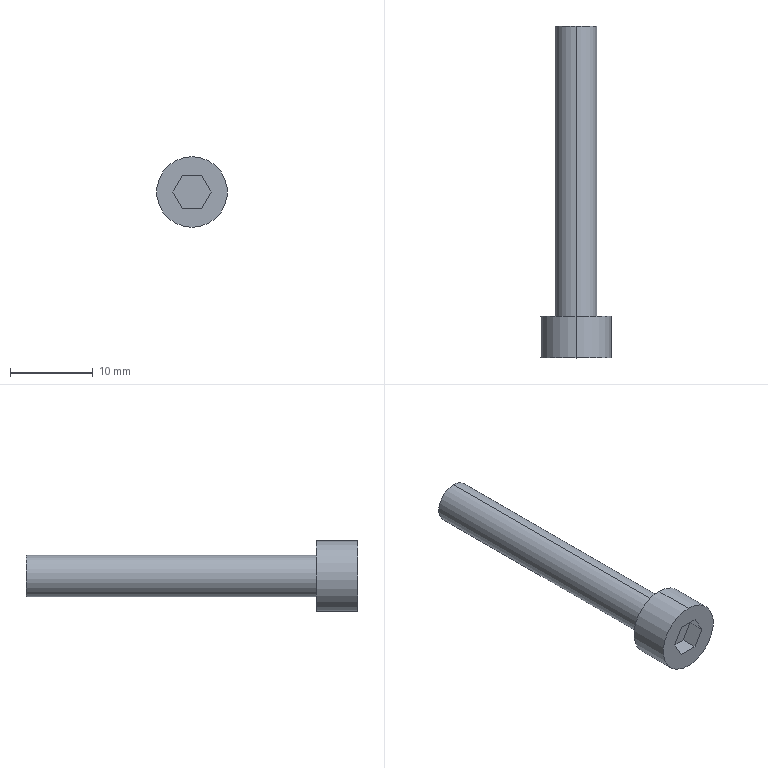Part | SolidWorks | features BaseBody 1 | 1 solid | 14 faces | box 8.5 x 40 x 8.5 mm | volume 943.236 mm3 | plane 10 | cylinder 4 | commonest cylinder face diameters 5 x2 8.5 x2
STEP:
#1=CARTESIAN_POINT('',(0.,40.,-2.5));
#2=VERTEX_POINT('',#1);
#3=CARTESIAN_POINT('',(0.,40.,2.5));
#4=VERTEX_POINT('',#3);
#5=CARTESIAN_POINT('',(0.,40.,0.));
#6=DIRECTION('',(0.,-1.,0.));
#7=DIRECTION('',(0.,0.,-1.));
#8=AXIS2_PLACEMENT_3D('',#5,#6,#7);
#9=CIRCLE('',#8,2.5);
#10=EDGE_CURVE('',#2,#4,#9,.T.);
#11=ORIENTED_EDGE('',*,*,#10,.T.);
#12=CARTESIAN_POINT('',(0.,5.,2.5));
#13=VERTEX_POINT('',#12);
#14=CARTESIAN_POINT('',(0.,40.,2.5));
#15=DIRECTION('',(0.,-1.,0.));
#16=VECTOR('',#15,1000.);
#17=LINE('',#14,#16);
#18=EDGE_CURVE('',#4,#13,#17,.T.);
#19=ORIENTED_EDGE('',*,*,#18,.T.);
#20=CARTESIAN_POINT('',(0.,5.,-2.5));
#21=VERTEX_POINT('',#20);
#22=CARTESIAN_POINT('',(0.,5.,0.));
#23=DIRECTION('',(0.,1.,0.));
#24=DIRECTION('',(0.,0.,-1.));
#25=AXIS2_PLACEMENT_3D('',#22,#23,#24);
#26=CIRCLE('',#25,2.5);
#27=EDGE_CURVE('',#13,#21,#26,.T.);
#28=ORIENTED_EDGE('',*,*,#27,.T.);
#29=CARTESIAN_POINT('',(0.,40.,-2.5));
#30=DIRECTION('',(0.,-1.,0.));
#31=VECTOR('',#30,1000.);
#32=LINE('',#29,#31);
#33=EDGE_CURVE('',#2,#21,#32,.T.);
#34=ORIENTED_EDGE('',*,*,#33,.F.);
#35=EDGE_LOOP('',(#11,#19,#28,#34));
#36=FACE_OUTER_BOUND('',#35,.T.);
#37=CARTESIAN_POINT('',(0.,40.,0.));
#38=DIRECTION('',(0.,-1.,0.));
#39=DIRECTION('',(0.,0.,-1.));
#40=AXIS2_PLACEMENT_3D('',#37,#38,#39);
#41=CYLINDRICAL_SURFACE('',#40,2.5);
#42=ADVANCED_FACE('',(#36),#41,.T.);
#43=CARTESIAN_POINT('',(0.,5.,4.25));
#44=VERTEX_POINT('',#43);
#45=CARTESIAN_POINT('',(0.,5.,-4.25));
#46=VERTEX_POINT('',#45);
#47=CARTESIAN_POINT('',(0.,5.,0.));
#48=DIRECTION('',(0.,1.,0.));
#49=DIRECTION('',(0.,0.,-1.));
#50=AXIS2_PLACEMENT_3D('',#47,#48,#49);
#51=CIRCLE('',#50,4.25);
#52=EDGE_CURVE('',#44,#46,#51,.T.);
#53=ORIENTED_EDGE('',*,*,#52,.F.);
#54=CARTESIAN_POINT('',(0.,0.,4.25));
#55=VERTEX_POINT('',#54);
#56=CARTESIAN_POINT('',(0.,5.,4.25));
#57=DIRECTION('',(0.,-1.,0.));
#58=VECTOR('',#57,1000.);
#59=LINE('',#56,#58);
#60=EDGE_CURVE('',#44,#55,#59,.T.);
#61=ORIENTED_EDGE('',*,*,#60,.T.);
#62=CARTESIAN_POINT('',(0.,0.,-4.25));
#63=VERTEX_POINT('',#62);
#64=CARTESIAN_POINT('',(0.,0.,0.));
#65=DIRECTION('',(0.,1.,0.));
#66=DIRECTION('',(0.,0.,-1.));
#67=AXIS2_PLACEMENT_3D('',#64,#65,#66);
#68=CIRCLE('',#67,4.25);
#69=EDGE_CURVE('',#55,#63,#68,.T.);
#70=ORIENTED_EDGE('',*,*,#69,.T.);
#71=CARTESIAN_POINT('',(0.,5.,-4.25));
#72=DIRECTION('',(0.,-1.,0.));
#73=VECTOR('',#72,1000.);
#74=LINE('',#71,#73);
#75=EDGE_CURVE('',#46,#63,#74,.T.);
#76=ORIENTED_EDGE('',*,*,#75,.F.);
#77=EDGE_LOOP('',(#53,#61,#70,#76));
#78=FACE_OUTER_BOUND('',#77,.T.);
#79=CARTESIAN_POINT('',(0.,5.,0.));
#80=DIRECTION('',(0.,-1.,0.));
#81=DIRECTION('',(0.,0.,-1.));
#82=AXIS2_PLACEMENT_3D('',#79,#80,#81);
#83=CYLINDRICAL_SURFACE('',#82,4.25);
#84=ADVANCED_FACE('',(#78),#83,.T.);
#85=ORIENTED_EDGE('',*,*,#18,.F.);
#86=CARTESIAN_POINT('',(0.,40.,0.));
#87=DIRECTION('',(0.,-1.,0.));
#88=DIRECTION('',(0.,0.,-1.));
#89=AXIS2_PLACEMENT_3D('',#86,#87,#88);
#90=CIRCLE('',#89,2.5);
#91=EDGE_CURVE('',#4,#2,#90,.T.);
#92=ORIENTED_EDGE('',*,*,#91,.T.);
#93=ORIENTED_EDGE('',*,*,#33,.T.);
#94=CARTESIAN_POINT('',(0.,5.,0.));
#95=DIRECTION('',(0.,1.,0.));
#96=DIRECTION('',(0.,0.,-1.));
#97=AXIS2_PLACEMENT_3D('',#94,#95,#96);
#98=CIRCLE('',#97,2.5);
#99=EDGE_CURVE('',#21,#13,#98,.T.);
#100=ORIENTED_EDGE('',*,*,#99,.T.);
#101=EDGE_LOOP('',(#85,#92,#93,#100));
#102=FACE_OUTER_BOUND('',#101,.T.);
#103=CARTESIAN_POINT('',(0.,40.,0.));
#104=DIRECTION('',(0.,-1.,0.));
#105=DIRECTION('',(0.,0.,-1.));
#106=AXIS2_PLACEMENT_3D('',#103,#104,#105);
#107=CYLINDRICAL_SURFACE('',#106,2.5);
#108=ADVANCED_FACE('',(#102),#107,.T.);
#109=CARTESIAN_POINT('',(0.,5.,0.));
#110=DIRECTION('',(0.,1.,0.));
#111=DIRECTION('',(0.,0.,-1.));
#112=AXIS2_PLACEMENT_3D('',#109,#110,#111);
#113=CIRCLE('',#112,4.25);
#114=EDGE_CURVE('',#46,#44,#113,.T.);
#115=ORIENTED_EDGE('',*,*,#114,.T.);
#116=ORIENTED_EDGE('',*,*,#52,.T.);
#117=EDGE_LOOP('',(#115,#116));
#118=FACE_OUTER_BOUND('',#117,.T.);
#119=ORIENTED_EDGE('',*,*,#99,.F.);
#120=ORIENTED_EDGE('',*,*,#27,.F.);
#121=EDGE_LOOP('',(#119,#120));
#122=FACE_BOUND('',#121,.T.);
#123=CARTESIAN_POINT('',(0.,5.,0.));
#124=DIRECTION('',(0.,1.,0.));
#125=DIRECTION('',(0.,0.,1.));
#126=AXIS2_PLACEMENT_3D('',#123,#124,#125);
#127=PLANE('',#126);
#128=ADVANCED_FACE('',(#118,#122),#127,.T.);
#129=ORIENTED_EDGE('',*,*,#10,.F.);
#130=ORIENTED_EDGE('',*,*,#91,.F.);
#131=EDGE_LOOP('',(#129,#130));
#132=FACE_OUTER_BOUND('',#131,.T.);
#133=CARTESIAN_POINT('',(0.,40.,0.));
#134=DIRECTION('',(0.,1.,0.));
#135=DIRECTION('',(0.,0.,1.));
#136=AXIS2_PLACEMENT_3D('',#133,#134,#135);
#137=PLANE('',#136);
#138=ADVANCED_FACE('',(#132),#137,.T.);
#139=ORIENTED_EDGE('',*,*,#60,.F.);
#140=ORIENTED_EDGE('',*,*,#114,.F.);
#141=ORIENTED_EDGE('',*,*,#75,.T.);
#142=CARTESIAN_POINT('',(0.,0.,0.));
#143=DIRECTION('',(0.,1.,0.));
#144=DIRECTION('',(0.,0.,-1.));
#145=AXIS2_PLACEMENT_3D('',#142,#143,#144);
#146=CIRCLE('',#145,4.25);
#147=EDGE_CURVE('',#63,#55,#146,.T.);
#148=ORIENTED_EDGE('',*,*,#147,.T.);
#149=EDGE_LOOP('',(#139,#140,#141,#148));
#150=FACE_OUTER_BOUND('',#149,.T.);
#151=CARTESIAN_POINT('',(0.,5.,0.));
#152=DIRECTION('',(0.,-1.,0.));
#153=DIRECTION('',(0.,0.,-1.));
#154=AXIS2_PLACEMENT_3D('',#151,#152,#153);
#155=CYLINDRICAL_SURFACE('',#154,4.25);
#156=ADVANCED_FACE('',(#150),#155,.T.);
#157=ORIENTED_EDGE('',*,*,#147,.F.);
#158=ORIENTED_EDGE('',*,*,#69,.F.);
#159=EDGE_LOOP('',(#157,#158));
#160=FACE_OUTER_BOUND('',#159,.T.);
#161=CARTESIAN_POINT('',(1.155,0.,-2.));
#162=VERTEX_POINT('',#161);
#163=CARTESIAN_POINT('',(2.309,0.,0.));
#164=VERTEX_POINT('',#163);
#165=CARTESIAN_POINT('',(1.155,0.,-2.));
#166=DIRECTION('',(0.5,0.,0.866));
#167=VECTOR('',#166,1000.);
#168=LINE('',#165,#167);
#169=EDGE_CURVE('',#162,#164,#168,.T.);
#170=ORIENTED_EDGE('',*,*,#169,.F.);
#171=CARTESIAN_POINT('',(-1.155,0.,-2.));
#172=VERTEX_POINT('',#171);
#173=CARTESIAN_POINT('',(0.,0.,-2.));
#174=DIRECTION('',(1.,0.,0.));
#175=VECTOR('',#174,1000.);
#176=LINE('',#173,#175);
#177=EDGE_CURVE('',#172,#162,#176,.T.);
#178=ORIENTED_EDGE('',*,*,#177,.F.);
#179=CARTESIAN_POINT('',(-2.309,0.,0.));
#180=VERTEX_POINT('',#179);
#181=CARTESIAN_POINT('',(-2.309,0.,0.));
#182=DIRECTION('',(0.5,0.,-0.866));
#183=VECTOR('',#182,1000.);
#184=LINE('',#181,#183);
#185=EDGE_CURVE('',#180,#172,#184,.T.);
#186=ORIENTED_EDGE('',*,*,#185,.F.);
#187=CARTESIAN_POINT('',(-1.155,0.,2.));
#188=VERTEX_POINT('',#187);
#189=CARTESIAN_POINT('',(-1.155,0.,2.));
#190=DIRECTION('',(-0.5,0.,-0.866));
#191=VECTOR('',#190,1000.);
#192=LINE('',#189,#191);
#193=EDGE_CURVE('',#188,#180,#192,.T.);
#194=ORIENTED_EDGE('',*,*,#193,.F.);
#195=CARTESIAN_POINT('',(1.155,0.,2.));
#196=VERTEX_POINT('',#195);
#197=CARTESIAN_POINT('',(0.,0.,2.));
#198=DIRECTION('',(-1.,0.,0.));
#199=VECTOR('',#198,1000.);
#200=LINE('',#197,#199);
#201=EDGE_CURVE('',#196,#188,#200,.T.);
#202=ORIENTED_EDGE('',*,*,#201,.F.);
#203=CARTESIAN_POINT('',(2.309,0.,0.));
#204=DIRECTION('',(-0.5,0.,0.866));
#205=VECTOR('',#204,1000.);
#206=LINE('',#203,#205);
#207=EDGE_CURVE('',#164,#196,#206,.T.);
#208=ORIENTED_EDGE('',*,*,#207,.F.);
#209=EDGE_LOOP('',(#170,#178,#186,#194,#202,#208));
#210=FACE_BOUND('',#209,.T.);
#211=CARTESIAN_POINT('',(0.,0.,0.));
#212=DIRECTION('',(0.,1.,0.));
#213=DIRECTION('',(0.,0.,1.));
#214=AXIS2_PLACEMENT_3D('',#211,#212,#213);
#215=PLANE('',#214);
#216=ADVANCED_FACE('',(#160,#210),#215,.F.);
#217=CARTESIAN_POINT('',(1.155,2.,2.));
#218=VERTEX_POINT('',#217);
#219=CARTESIAN_POINT('',(1.155,2.,2.));
#220=DIRECTION('',(0.,-1.,0.));
#221=VECTOR('',#220,1000.);
#222=LINE('',#219,#221);
#223=EDGE_CURVE('',#218,#196,#222,.T.);
#224=ORIENTED_EDGE('',*,*,#223,.F.);
#225=CARTESIAN_POINT('',(2.309,2.,0.));
#226=VERTEX_POINT('',#225);
#227=CARTESIAN_POINT('',(2.309,2.,0.));
#228=DIRECTION('',(-0.5,0.,0.866));
#229=VECTOR('',#228,1000.);
#230=LINE('',#227,#229);
#231=EDGE_CURVE('',#226,#218,#230,.T.);
#232=ORIENTED_EDGE('',*,*,#231,.F.);
#233=CARTESIAN_POINT('',(2.309,2.,0.));
#234=DIRECTION('',(0.,1.,0.));
#235=VECTOR('',#234,1000.);
#236=LINE('',#233,#235);
#237=EDGE_CURVE('',#164,#226,#236,.T.);
#238=ORIENTED_EDGE('',*,*,#237,.F.);
#239=ORIENTED_EDGE('',*,*,#207,.T.);
#240=EDGE_LOOP('',(#224,#232,#238,#239));
#241=FACE_OUTER_BOUND('',#240,.T.);
#242=CARTESIAN_POINT('',(2.309,2.,0.));
#243=DIRECTION('',(0.866,0.,0.5));
#244=DIRECTION('',(0.5,0.,-0.866));
#245=AXIS2_PLACEMENT_3D('',#242,#243,#244);
#246=PLANE('',#245);
#247=ADVANCED_FACE('',(#241),#246,.F.);
#248=ORIENTED_EDGE('',*,*,#237,.T.);
#249=CARTESIAN_POINT('',(1.155,2.,-2.));
#250=VERTEX_POINT('',#249);
#251=CARTESIAN_POINT('',(1.155,2.,-2.));
#252=DIRECTION('',(0.5,0.,0.866));
#253=VECTOR('',#252,1000.);
#254=LINE('',#251,#253);
#255=EDGE_CURVE('',#250,#226,#254,.T.);
#256=ORIENTED_EDGE('',*,*,#255,.F.);
#257=CARTESIAN_POINT('',(1.155,2.,-2.));
#258=DIRECTION('',(0.,1.,0.));
#259=VECTOR('',#258,1000.);
#260=LINE('',#257,#259);
#261=EDGE_CURVE('',#162,#250,#260,.T.);
#262=ORIENTED_EDGE('',*,*,#261,.F.);
#263=ORIENTED_EDGE('',*,*,#169,.T.);
#264=EDGE_LOOP('',(#248,#256,#262,#263));
#265=FACE_OUTER_BOUND('',#264,.T.);
#266=CARTESIAN_POINT('',(1.155,2.,-2.));
#267=DIRECTION('',(0.866,0.,-0.5));
#268=DIRECTION('',(-0.5,0.,-0.866));
#269=AXIS2_PLACEMENT_3D('',#266,#267,#268);
#270=PLANE('',#269);
#271=ADVANCED_FACE('',(#265),#270,.F.);
#272=ORIENTED_EDGE('',*,*,#261,.T.);
#273=CARTESIAN_POINT('',(-1.155,2.,-2.));
#274=VERTEX_POINT('',#273);
#275=CARTESIAN_POINT('',(-1.155,2.,-2.));
#276=DIRECTION('',(1.,0.,0.));
#277=VECTOR('',#276,1000.);
#278=LINE('',#275,#277);
#279=EDGE_CURVE('',#274,#250,#278,.T.);
#280=ORIENTED_EDGE('',*,*,#279,.F.);
#281=CARTESIAN_POINT('',(-1.155,2.,-2.));
#282=DIRECTION('',(0.,1.,0.));
#283=VECTOR('',#282,1000.);
#284=LINE('',#281,#283);
#285=EDGE_CURVE('',#172,#274,#284,.T.);
#286=ORIENTED_EDGE('',*,*,#285,.F.);
#287=ORIENTED_EDGE('',*,*,#177,.T.);
#288=EDGE_LOOP('',(#272,#280,#286,#287));
#289=FACE_OUTER_BOUND('',#288,.T.);
#290=CARTESIAN_POINT('',(-1.155,2.,-2.));
#291=DIRECTION('',(0.,0.,-1.));
#292=DIRECTION('',(-1.,0.,0.));
#293=AXIS2_PLACEMENT_3D('',#290,#291,#292);
#294=PLANE('',#293);
#295=ADVANCED_FACE('',(#289),#294,.F.);
#296=ORIENTED_EDGE('',*,*,#285,.T.);
#297=CARTESIAN_POINT('',(-2.309,2.,0.));
#298=VERTEX_POINT('',#297);
#299=CARTESIAN_POINT('',(-2.309,2.,0.));
#300=DIRECTION('',(0.5,0.,-0.866));
#301=VECTOR('',#300,1000.);
#302=LINE('',#299,#301);
#303=EDGE_CURVE('',#298,#274,#302,.T.);
#304=ORIENTED_EDGE('',*,*,#303,.F.);
#305=CARTESIAN_POINT('',(-2.309,2.,0.));
#306=DIRECTION('',(0.,1.,0.));
#307=VECTOR('',#306,1000.);
#308=LINE('',#305,#307);
#309=EDGE_CURVE('',#180,#298,#308,.T.);
#310=ORIENTED_EDGE('',*,*,#309,.F.);
#311=ORIENTED_EDGE('',*,*,#185,.T.);
#312=EDGE_LOOP('',(#296,#304,#310,#311));
#313=FACE_OUTER_BOUND('',#312,.T.);
#314=CARTESIAN_POINT('',(-2.309,2.,0.));
#315=DIRECTION('',(-0.866,0.,-0.5));
#316=DIRECTION('',(-0.5,0.,0.866));
#317=AXIS2_PLACEMENT_3D('',#314,#315,#316);
#318=PLANE('',#317);
#319=ADVANCED_FACE('',(#313),#318,.F.);
#320=ORIENTED_EDGE('',*,*,#309,.T.);
#321=CARTESIAN_POINT('',(-1.155,2.,2.));
#322=VERTEX_POINT('',#321);
#323=CARTESIAN_POINT('',(-1.155,2.,2.));
#324=DIRECTION('',(-0.5,0.,-0.866));
#325=VECTOR('',#324,1000.);
#326=LINE('',#323,#325);
#327=EDGE_CURVE('',#322,#298,#326,.T.);
#328=ORIENTED_EDGE('',*,*,#327,.F.);
#329=CARTESIAN_POINT('',(-1.155,2.,2.));
#330=DIRECTION('',(0.,1.,0.));
#331=VECTOR('',#330,1000.);
#332=LINE('',#329,#331);
#333=EDGE_CURVE('',#188,#322,#332,.T.);
#334=ORIENTED_EDGE('',*,*,#333,.F.);
#335=ORIENTED_EDGE('',*,*,#193,.T.);
#336=EDGE_LOOP('',(#320,#328,#334,#335));
#337=FACE_OUTER_BOUND('',#336,.T.);
#338=CARTESIAN_POINT('',(-1.155,2.,2.));
#339=DIRECTION('',(-0.866,0.,0.5));
#340=DIRECTION('',(0.5,0.,0.866));
#341=AXIS2_PLACEMENT_3D('',#338,#339,#340);
#342=PLANE('',#341);
#343=ADVANCED_FACE('',(#337),#342,.F.);
#344=ORIENTED_EDGE('',*,*,#333,.T.);
#345=CARTESIAN_POINT('',(1.155,2.,2.));
#346=DIRECTION('',(-1.,0.,0.));
#347=VECTOR('',#346,1000.);
#348=LINE('',#345,#347);
#349=EDGE_CURVE('',#218,#322,#348,.T.);
#350=ORIENTED_EDGE('',*,*,#349,.F.);
#351=ORIENTED_EDGE('',*,*,#223,.T.);
#352=ORIENTED_EDGE('',*,*,#201,.T.);
#353=EDGE_LOOP('',(#344,#350,#351,#352));
#354=FACE_OUTER_BOUND('',#353,.T.);
#355=CARTESIAN_POINT('',(1.155,2.,2.));
#356=DIRECTION('',(0.,0.,1.));
#357=DIRECTION('',(1.,0.,0.));
#358=AXIS2_PLACEMENT_3D('',#355,#356,#357);
#359=PLANE('',#358);
#360=ADVANCED_FACE('',(#354),#359,.F.);
#361=ORIENTED_EDGE('',*,*,#303,.T.);
#362=ORIENTED_EDGE('',*,*,#279,.T.);
#363=ORIENTED_EDGE('',*,*,#255,.T.);
#364=ORIENTED_EDGE('',*,*,#231,.T.);
#365=ORIENTED_EDGE('',*,*,#349,.T.);
#366=ORIENTED_EDGE('',*,*,#327,.T.);
#367=EDGE_LOOP('',(#361,#362,#363,#364,#365,#366));
#368=FACE_OUTER_BOUND('',#367,.T.);
#369=CARTESIAN_POINT('',(0.,2.,0.));
#370=DIRECTION('',(0.,-1.,0.));
#371=DIRECTION('',(0.,0.,-1.));
#372=AXIS2_PLACEMENT_3D('',#369,#370,#371);
#373=PLANE('',#372);
#374=ADVANCED_FACE('',(#368),#373,.T.);
#375=CLOSED_SHELL('',(#42,#84,#108,#128,#138,#156,#216,#247,#271,#295,#319,#343,#360,#374));
#376=MANIFOLD_SOLID_BREP('',#375);
#377=CARTESIAN_POINT('',(0.,0.,0.));
#378=DIRECTION('',(0.,0.,1.));
#379=DIRECTION('',(1.,0.,0.));
#380=AXIS2_PLACEMENT_3D('',#377,#378,#379);
#381=(LENGTH_UNIT()NAMED_UNIT(*)SI_UNIT(.MILLI.,.METRE.));
#382=UNCERTAINTY_MEASURE_WITH_UNIT(LENGTH_MEASURE(0.00001),#381,'','');
#383=(NAMED_UNIT(*)PLANE_ANGLE_UNIT()SI_UNIT($,.RADIAN.));
#384=(NAMED_UNIT(*)SI_UNIT($,.STERADIAN.)SOLID_ANGLE_UNIT());
#385=(GEOMETRIC_REPRESENTATION_CONTEXT(3)GLOBAL_UNCERTAINTY_ASSIGNED_CONTEXT((#382))GLOBAL_UNIT_ASSIGNED_CONTEXT((#381,#383,#384))REPRESENTATION_CONTEXT('',''));
#386=ADVANCED_BREP_SHAPE_REPRESENTATION('',(#376,#380),#385);